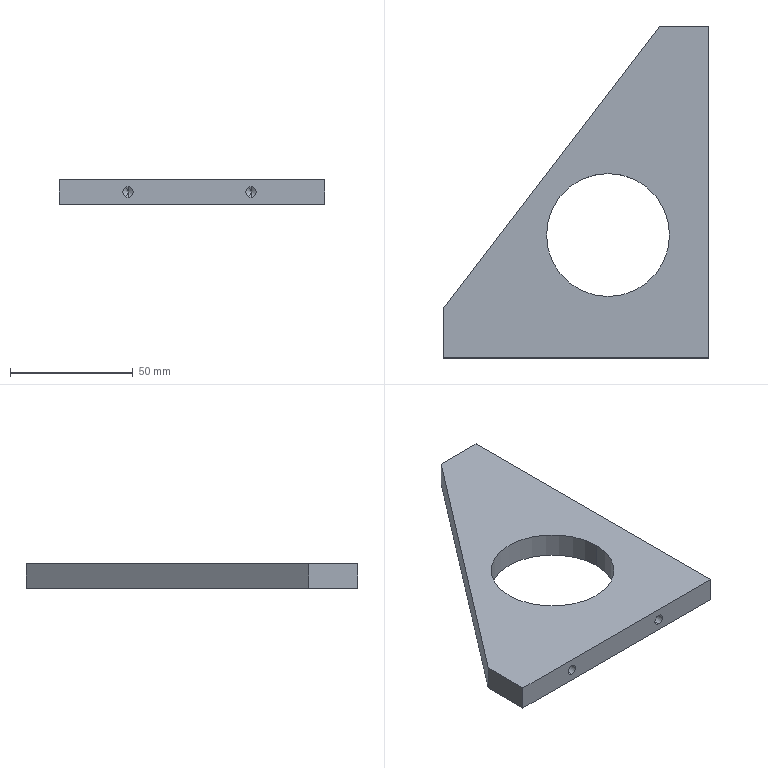Part | SolidWorks | features HoleWzd 2, ICE 2, Extrusion 1 | 1 solid | 25 faces | box 108 x 135 x 10 mm | volume 74855 mm3 | cylinder 10 | cone 8 | plane 7 | commonest cylinder face diameters 4.2 x8 50 x2
STEP:
#1=CARTESIAN_POINT('',(38.028,-17.5,10.));
#2=VERTEX_POINT('',#1);
#3=CARTESIAN_POINT('',(-11.972,-17.5,10.));
#4=VERTEX_POINT('',#3);
#5=CARTESIAN_POINT('',(13.028,-17.5,10.));
#6=DIRECTION('',(0.,0.,-1.));
#7=DIRECTION('',(1.,0.,0.));
#8=AXIS2_PLACEMENT_3D('',#5,#6,#7);
#9=CIRCLE('',#8,25.);
#10=EDGE_CURVE('',#2,#4,#9,.T.);
#11=ORIENTED_EDGE('',*,*,#10,.F.);
#12=CARTESIAN_POINT('',(38.028,-17.5,0.));
#13=VERTEX_POINT('',#12);
#14=CARTESIAN_POINT('',(38.028,-17.5,10.001));
#15=DIRECTION('',(0.,0.,-1.));
#16=VECTOR('',#15,1000.);
#17=LINE('',#14,#16);
#18=EDGE_CURVE('',#2,#13,#17,.T.);
#19=ORIENTED_EDGE('',*,*,#18,.T.);
#20=CARTESIAN_POINT('',(-11.972,-17.5,0.));
#21=VERTEX_POINT('',#20);
#22=CARTESIAN_POINT('',(13.028,-17.5,0.));
#23=DIRECTION('',(0.,0.,-1.));
#24=DIRECTION('',(-1.,0.,0.));
#25=AXIS2_PLACEMENT_3D('',#22,#23,#24);
#26=CIRCLE('',#25,25.);
#27=EDGE_CURVE('',#13,#21,#26,.T.);
#28=ORIENTED_EDGE('',*,*,#27,.T.);
#29=CARTESIAN_POINT('',(-11.972,-17.5,10.001));
#30=DIRECTION('',(0.,0.,-1.));
#31=VECTOR('',#30,1000.);
#32=LINE('',#29,#31);
#33=EDGE_CURVE('',#4,#21,#32,.T.);
#34=ORIENTED_EDGE('',*,*,#33,.F.);
#35=EDGE_LOOP('',(#11,#19,#28,#34));
#36=FACE_OUTER_BOUND('',#35,.T.);
#37=CARTESIAN_POINT('',(13.028,-17.5,10.001));
#38=DIRECTION('',(0.,0.,-1.));
#39=DIRECTION('',(-1.,0.,0.));
#40=AXIS2_PLACEMENT_3D('',#37,#38,#39);
#41=CYLINDRICAL_SURFACE('',#40,25.);
#42=ADVANCED_FACE('',(#36),#41,.F.);
#43=CARTESIAN_POINT('',(41.6,-27.5,7.1));
#44=VERTEX_POINT('',#43);
#45=CARTESIAN_POINT('',(41.6,-27.5,2.9));
#46=VERTEX_POINT('',#45);
#47=CARTESIAN_POINT('',(41.6,-27.5,5.));
#48=DIRECTION('',(1.,0.,0.));
#49=DIRECTION('',(0.,0.,-1.));
#50=AXIS2_PLACEMENT_3D('',#47,#48,#49);
#51=CIRCLE('',#50,2.1);
#52=EDGE_CURVE('',#44,#46,#51,.T.);
#53=ORIENTED_EDGE('',*,*,#52,.F.);
#54=CARTESIAN_POINT('',(54.,-27.5,7.1));
#55=VERTEX_POINT('',#54);
#56=CARTESIAN_POINT('',(54.,-27.5,7.1));
#57=DIRECTION('',(1.,0.,0.));
#58=VECTOR('',#57,1000.);
#59=LINE('',#56,#58);
#60=EDGE_CURVE('',#44,#55,#59,.T.);
#61=ORIENTED_EDGE('',*,*,#60,.T.);
#62=CARTESIAN_POINT('',(54.,-27.5,2.9));
#63=VERTEX_POINT('',#62);
#64=CARTESIAN_POINT('',(54.,-27.5,5.));
#65=DIRECTION('',(1.,0.,0.));
#66=DIRECTION('',(0.,0.,-1.));
#67=AXIS2_PLACEMENT_3D('',#64,#65,#66);
#68=CIRCLE('',#67,2.1);
#69=EDGE_CURVE('',#55,#63,#68,.T.);
#70=ORIENTED_EDGE('',*,*,#69,.T.);
#71=CARTESIAN_POINT('',(54.,-27.5,2.9));
#72=DIRECTION('',(1.,0.,0.));
#73=VECTOR('',#72,1000.);
#74=LINE('',#71,#73);
#75=EDGE_CURVE('',#46,#63,#74,.T.);
#76=ORIENTED_EDGE('',*,*,#75,.F.);
#77=EDGE_LOOP('',(#53,#61,#70,#76));
#78=FACE_OUTER_BOUND('',#77,.T.);
#79=CARTESIAN_POINT('',(54.,-27.5,5.));
#80=DIRECTION('',(1.,0.,0.));
#81=DIRECTION('',(0.,0.,-1.));
#82=AXIS2_PLACEMENT_3D('',#79,#80,#81);
#83=CYLINDRICAL_SURFACE('',#82,2.1);
#84=ADVANCED_FACE('',(#78),#83,.F.);
#85=CARTESIAN_POINT('',(40.338,-27.5,5.));
#86=VERTEX_POINT('',#85);
#87=CARTESIAN_POINT('',(41.6,-27.5,2.9));
#88=DIRECTION('',(0.515,0.,-0.8572));
#89=VECTOR('',#88,1000.);
#90=LINE('',#87,#89);
#91=EDGE_CURVE('',#86,#46,#90,.T.);
#92=ORIENTED_EDGE('',*,*,#91,.F.);
#93=CARTESIAN_POINT('',(41.6,-27.5,7.1));
#94=DIRECTION('',(0.515,0.,0.8572));
#95=VECTOR('',#94,1000.);
#96=LINE('',#93,#95);
#97=EDGE_CURVE('',#86,#44,#96,.T.);
#98=ORIENTED_EDGE('',*,*,#97,.T.);
#99=ORIENTED_EDGE('',*,*,#52,.T.);
#100=EDGE_LOOP('',(#92,#98,#99));
#101=FACE_OUTER_BOUND('',#100,.T.);
#102=CARTESIAN_POINT('',(41.6,-27.5,5.));
#103=DIRECTION('',(1.,0.,0.));
#104=DIRECTION('',(0.,0.,-1.));
#105=AXIS2_PLACEMENT_3D('',#102,#103,#104);
#106=CONICAL_SURFACE('',#105,2.1,1.03);
#107=ADVANCED_FACE('',(#101),#106,.F.);
#108=CARTESIAN_POINT('',(41.6,32.5,7.1));
#109=VERTEX_POINT('',#108);
#110=CARTESIAN_POINT('',(41.6,32.5,2.9));
#111=VERTEX_POINT('',#110);
#112=CARTESIAN_POINT('',(41.6,32.5,5.));
#113=DIRECTION('',(1.,0.,0.));
#114=DIRECTION('',(0.,0.,-1.));
#115=AXIS2_PLACEMENT_3D('',#112,#113,#114);
#116=CIRCLE('',#115,2.1);
#117=EDGE_CURVE('',#109,#111,#116,.T.);
#118=ORIENTED_EDGE('',*,*,#117,.F.);
#119=CARTESIAN_POINT('',(54.,32.5,7.1));
#120=VERTEX_POINT('',#119);
#121=CARTESIAN_POINT('',(54.,32.5,7.1));
#122=DIRECTION('',(1.,0.,0.));
#123=VECTOR('',#122,1000.);
#124=LINE('',#121,#123);
#125=EDGE_CURVE('',#109,#120,#124,.T.);
#126=ORIENTED_EDGE('',*,*,#125,.T.);
#127=CARTESIAN_POINT('',(54.,32.5,2.9));
#128=VERTEX_POINT('',#127);
#129=CARTESIAN_POINT('',(54.,32.5,5.));
#130=DIRECTION('',(1.,0.,0.));
#131=DIRECTION('',(0.,0.,-1.));
#132=AXIS2_PLACEMENT_3D('',#129,#130,#131);
#133=CIRCLE('',#132,2.1);
#134=EDGE_CURVE('',#120,#128,#133,.T.);
#135=ORIENTED_EDGE('',*,*,#134,.T.);
#136=CARTESIAN_POINT('',(54.,32.5,2.9));
#137=DIRECTION('',(1.,0.,0.));
#138=VECTOR('',#137,1000.);
#139=LINE('',#136,#138);
#140=EDGE_CURVE('',#111,#128,#139,.T.);
#141=ORIENTED_EDGE('',*,*,#140,.F.);
#142=EDGE_LOOP('',(#118,#126,#135,#141));
#143=FACE_OUTER_BOUND('',#142,.T.);
#144=CARTESIAN_POINT('',(54.,32.5,5.));
#145=DIRECTION('',(1.,0.,0.));
#146=DIRECTION('',(0.,0.,-1.));
#147=AXIS2_PLACEMENT_3D('',#144,#145,#146);
#148=CYLINDRICAL_SURFACE('',#147,2.1);
#149=ADVANCED_FACE('',(#143),#148,.F.);
#150=CARTESIAN_POINT('',(40.338,32.5,5.));
#151=VERTEX_POINT('',#150);
#152=CARTESIAN_POINT('',(41.6,32.5,2.9));
#153=DIRECTION('',(0.515,0.,-0.8572));
#154=VECTOR('',#153,1000.);
#155=LINE('',#152,#154);
#156=EDGE_CURVE('',#151,#111,#155,.T.);
#157=ORIENTED_EDGE('',*,*,#156,.F.);
#158=CARTESIAN_POINT('',(41.6,32.5,7.1));
#159=DIRECTION('',(0.515,0.,0.8572));
#160=VECTOR('',#159,1000.);
#161=LINE('',#158,#160);
#162=EDGE_CURVE('',#151,#109,#161,.T.);
#163=ORIENTED_EDGE('',*,*,#162,.T.);
#164=ORIENTED_EDGE('',*,*,#117,.T.);
#165=EDGE_LOOP('',(#157,#163,#164));
#166=FACE_OUTER_BOUND('',#165,.T.);
#167=CARTESIAN_POINT('',(41.6,32.5,5.));
#168=DIRECTION('',(1.,0.,0.));
#169=DIRECTION('',(0.,0.,-1.));
#170=AXIS2_PLACEMENT_3D('',#167,#168,#169);
#171=CONICAL_SURFACE('',#170,2.1,1.03);
#172=ADVANCED_FACE('',(#166),#171,.F.);
#173=CARTESIAN_POINT('',(24.,-55.1,7.1));
#174=VERTEX_POINT('',#173);
#175=CARTESIAN_POINT('',(24.,-55.1,2.9));
#176=VERTEX_POINT('',#175);
#177=CARTESIAN_POINT('',(24.,-55.1,5.));
#178=DIRECTION('',(0.,-1.,0.));
#179=DIRECTION('',(0.,0.,-1.));
#180=AXIS2_PLACEMENT_3D('',#177,#178,#179);
#181=CIRCLE('',#180,2.1);
#182=EDGE_CURVE('',#174,#176,#181,.T.);
#183=ORIENTED_EDGE('',*,*,#182,.F.);
#184=CARTESIAN_POINT('',(24.,-67.5,7.1));
#185=VERTEX_POINT('',#184);
#186=CARTESIAN_POINT('',(24.,-67.5,7.1));
#187=DIRECTION('',(0.,-1.,0.));
#188=VECTOR('',#187,1000.);
#189=LINE('',#186,#188);
#190=EDGE_CURVE('',#174,#185,#189,.T.);
#191=ORIENTED_EDGE('',*,*,#190,.T.);
#192=CARTESIAN_POINT('',(24.,-67.5,2.9));
#193=VERTEX_POINT('',#192);
#194=CARTESIAN_POINT('',(24.,-67.5,5.));
#195=DIRECTION('',(0.,-1.,0.));
#196=DIRECTION('',(0.,0.,-1.));
#197=AXIS2_PLACEMENT_3D('',#194,#195,#196);
#198=CIRCLE('',#197,2.1);
#199=EDGE_CURVE('',#185,#193,#198,.T.);
#200=ORIENTED_EDGE('',*,*,#199,.T.);
#201=CARTESIAN_POINT('',(24.,-67.5,2.9));
#202=DIRECTION('',(0.,-1.,0.));
#203=VECTOR('',#202,1000.);
#204=LINE('',#201,#203);
#205=EDGE_CURVE('',#176,#193,#204,.T.);
#206=ORIENTED_EDGE('',*,*,#205,.F.);
#207=EDGE_LOOP('',(#183,#191,#200,#206));
#208=FACE_OUTER_BOUND('',#207,.T.);
#209=CARTESIAN_POINT('',(24.,-67.5,5.));
#210=DIRECTION('',(0.,-1.,0.));
#211=DIRECTION('',(0.,0.,-1.));
#212=AXIS2_PLACEMENT_3D('',#209,#210,#211);
#213=CYLINDRICAL_SURFACE('',#212,2.1);
#214=ADVANCED_FACE('',(#208),#213,.F.);
#215=CARTESIAN_POINT('',(24.,-53.838,5.));
#216=VERTEX_POINT('',#215);
#217=CARTESIAN_POINT('',(24.,-55.1,2.9));
#218=DIRECTION('',(0.,-0.515,-0.8572));
#219=VECTOR('',#218,1000.);
#220=LINE('',#217,#219);
#221=EDGE_CURVE('',#216,#176,#220,.T.);
#222=ORIENTED_EDGE('',*,*,#221,.F.);
#223=CARTESIAN_POINT('',(24.,-55.1,7.1));
#224=DIRECTION('',(0.,-0.515,0.8572));
#225=VECTOR('',#224,1000.);
#226=LINE('',#223,#225);
#227=EDGE_CURVE('',#216,#174,#226,.T.);
#228=ORIENTED_EDGE('',*,*,#227,.T.);
#229=ORIENTED_EDGE('',*,*,#182,.T.);
#230=EDGE_LOOP('',(#222,#228,#229));
#231=FACE_OUTER_BOUND('',#230,.T.);
#232=CARTESIAN_POINT('',(24.,-55.1,5.));
#233=DIRECTION('',(0.,-1.,0.));
#234=DIRECTION('',(0.,0.,-1.));
#235=AXIS2_PLACEMENT_3D('',#232,#233,#234);
#236=CONICAL_SURFACE('',#235,2.1,1.03);
#237=ADVANCED_FACE('',(#231),#236,.F.);
#238=CARTESIAN_POINT('',(-26.,-55.1,7.1));
#239=VERTEX_POINT('',#238);
#240=CARTESIAN_POINT('',(-26.,-55.1,2.9));
#241=VERTEX_POINT('',#240);
#242=CARTESIAN_POINT('',(-26.,-55.1,5.));
#243=DIRECTION('',(0.,-1.,0.));
#244=DIRECTION('',(0.,0.,-1.));
#245=AXIS2_PLACEMENT_3D('',#242,#243,#244);
#246=CIRCLE('',#245,2.1);
#247=EDGE_CURVE('',#239,#241,#246,.T.);
#248=ORIENTED_EDGE('',*,*,#247,.F.);
#249=CARTESIAN_POINT('',(-26.,-67.5,7.1));
#250=VERTEX_POINT('',#249);
#251=CARTESIAN_POINT('',(-26.,-67.5,7.1));
#252=DIRECTION('',(0.,-1.,0.));
#253=VECTOR('',#252,1000.);
#254=LINE('',#251,#253);
#255=EDGE_CURVE('',#239,#250,#254,.T.);
#256=ORIENTED_EDGE('',*,*,#255,.T.);
#257=CARTESIAN_POINT('',(-26.,-67.5,2.9));
#258=VERTEX_POINT('',#257);
#259=CARTESIAN_POINT('',(-26.,-67.5,5.));
#260=DIRECTION('',(0.,-1.,0.));
#261=DIRECTION('',(0.,0.,-1.));
#262=AXIS2_PLACEMENT_3D('',#259,#260,#261);
#263=CIRCLE('',#262,2.1);
#264=EDGE_CURVE('',#250,#258,#263,.T.);
#265=ORIENTED_EDGE('',*,*,#264,.T.);
#266=CARTESIAN_POINT('',(-26.,-67.5,2.9));
#267=DIRECTION('',(0.,-1.,0.));
#268=VECTOR('',#267,1000.);
#269=LINE('',#266,#268);
#270=EDGE_CURVE('',#241,#258,#269,.T.);
#271=ORIENTED_EDGE('',*,*,#270,.F.);
#272=EDGE_LOOP('',(#248,#256,#265,#271));
#273=FACE_OUTER_BOUND('',#272,.T.);
#274=CARTESIAN_POINT('',(-26.,-67.5,5.));
#275=DIRECTION('',(0.,-1.,0.));
#276=DIRECTION('',(0.,0.,-1.));
#277=AXIS2_PLACEMENT_3D('',#274,#275,#276);
#278=CYLINDRICAL_SURFACE('',#277,2.1);
#279=ADVANCED_FACE('',(#273),#278,.F.);
#280=CARTESIAN_POINT('',(-26.,-53.838,5.));
#281=VERTEX_POINT('',#280);
#282=CARTESIAN_POINT('',(-26.,-55.1,2.9));
#283=DIRECTION('',(0.,-0.515,-0.8572));
#284=VECTOR('',#283,1000.);
#285=LINE('',#282,#284);
#286=EDGE_CURVE('',#281,#241,#285,.T.);
#287=ORIENTED_EDGE('',*,*,#286,.F.);
#288=CARTESIAN_POINT('',(-26.,-55.1,7.1));
#289=DIRECTION('',(0.,-0.515,0.8572));
#290=VECTOR('',#289,1000.);
#291=LINE('',#288,#290);
#292=EDGE_CURVE('',#281,#239,#291,.T.);
#293=ORIENTED_EDGE('',*,*,#292,.T.);
#294=ORIENTED_EDGE('',*,*,#247,.T.);
#295=EDGE_LOOP('',(#287,#293,#294));
#296=FACE_OUTER_BOUND('',#295,.T.);
#297=CARTESIAN_POINT('',(-26.,-55.1,5.));
#298=DIRECTION('',(0.,-1.,0.));
#299=DIRECTION('',(0.,0.,-1.));
#300=AXIS2_PLACEMENT_3D('',#297,#298,#299);
#301=CONICAL_SURFACE('',#300,2.1,1.03);
#302=ADVANCED_FACE('',(#296),#301,.F.);
#303=CARTESIAN_POINT('',(-54.,-47.5,10.));
#304=VERTEX_POINT('',#303);
#305=CARTESIAN_POINT('',(-54.,-67.5,10.));
#306=VERTEX_POINT('',#305);
#307=CARTESIAN_POINT('',(-54.,-67.5,10.));
#308=DIRECTION('',(0.,-1.,0.));
#309=VECTOR('',#308,1000.);
#310=LINE('',#307,#309);
#311=EDGE_CURVE('',#304,#306,#310,.T.);
#312=ORIENTED_EDGE('',*,*,#311,.F.);
#313=CARTESIAN_POINT('',(-54.,-47.5,0.));
#314=VERTEX_POINT('',#313);
#315=CARTESIAN_POINT('',(-54.,-47.5,-0.001));
#316=DIRECTION('',(0.,0.,1.));
#317=VECTOR('',#316,1000.);
#318=LINE('',#315,#317);
#319=EDGE_CURVE('',#314,#304,#318,.T.);
#320=ORIENTED_EDGE('',*,*,#319,.F.);
#321=CARTESIAN_POINT('',(-54.,-67.5,0.));
#322=VERTEX_POINT('',#321);
#323=CARTESIAN_POINT('',(-54.,-67.5,0.));
#324=DIRECTION('',(0.,-1.,0.));
#325=VECTOR('',#324,1000.);
#326=LINE('',#323,#325);
#327=EDGE_CURVE('',#314,#322,#326,.T.);
#328=ORIENTED_EDGE('',*,*,#327,.T.);
#329=CARTESIAN_POINT('',(-54.,-67.5,10.));
#330=DIRECTION('',(0.,0.,-1.));
#331=VECTOR('',#330,1000.);
#332=LINE('',#329,#331);
#333=EDGE_CURVE('',#306,#322,#332,.T.);
#334=ORIENTED_EDGE('',*,*,#333,.F.);
#335=EDGE_LOOP('',(#312,#320,#328,#334));
#336=FACE_OUTER_BOUND('',#335,.T.);
#337=CARTESIAN_POINT('',(-54.,-67.5,10.));
#338=DIRECTION('',(1.,0.,0.));
#339=DIRECTION('',(0.,0.,-1.));
#340=AXIS2_PLACEMENT_3D('',#337,#338,#339);
#341=PLANE('',#340);
#342=ADVANCED_FACE('',(#336),#341,.F.);
#343=CARTESIAN_POINT('',(24.,-67.5,5.));
#344=DIRECTION('',(0.,-1.,0.));
#345=DIRECTION('',(0.,0.,-1.));
#346=AXIS2_PLACEMENT_3D('',#343,#344,#345);
#347=CIRCLE('',#346,2.1);
#348=EDGE_CURVE('',#193,#185,#347,.T.);
#349=ORIENTED_EDGE('',*,*,#348,.F.);
#350=ORIENTED_EDGE('',*,*,#199,.F.);
#351=EDGE_LOOP('',(#349,#350));
#352=FACE_BOUND('',#351,.T.);
#353=CARTESIAN_POINT('',(-26.,-67.5,5.));
#354=DIRECTION('',(0.,-1.,0.));
#355=DIRECTION('',(0.,0.,-1.));
#356=AXIS2_PLACEMENT_3D('',#353,#354,#355);
#357=CIRCLE('',#356,2.1);
#358=EDGE_CURVE('',#258,#250,#357,.T.);
#359=ORIENTED_EDGE('',*,*,#358,.F.);
#360=ORIENTED_EDGE('',*,*,#264,.F.);
#361=EDGE_LOOP('',(#359,#360));
#362=FACE_BOUND('',#361,.T.);
#363=CARTESIAN_POINT('',(54.,-67.5,0.));
#364=VERTEX_POINT('',#363);
#365=CARTESIAN_POINT('',(54.,-67.5,0.));
#366=DIRECTION('',(1.,0.,0.));
#367=VECTOR('',#366,1000.);
#368=LINE('',#365,#367);
#369=EDGE_CURVE('',#322,#364,#368,.T.);
#370=ORIENTED_EDGE('',*,*,#369,.T.);
#371=CARTESIAN_POINT('',(54.,-67.5,10.));
#372=VERTEX_POINT('',#371);
#373=CARTESIAN_POINT('',(54.,-67.5,10.));
#374=DIRECTION('',(0.,0.,-1.));
#375=VECTOR('',#374,1000.);
#376=LINE('',#373,#375);
#377=EDGE_CURVE('',#372,#364,#376,.T.);
#378=ORIENTED_EDGE('',*,*,#377,.F.);
#379=CARTESIAN_POINT('',(54.,-67.5,10.));
#380=DIRECTION('',(1.,0.,0.));
#381=VECTOR('',#380,1000.);
#382=LINE('',#379,#381);
#383=EDGE_CURVE('',#306,#372,#382,.T.);
#384=ORIENTED_EDGE('',*,*,#383,.F.);
#385=ORIENTED_EDGE('',*,*,#333,.T.);
#386=EDGE_LOOP('',(#370,#378,#384,#385));
#387=FACE_OUTER_BOUND('',#386,.T.);
#388=CARTESIAN_POINT('',(54.,-67.5,10.));
#389=DIRECTION('',(0.,1.,0.));
#390=DIRECTION('',(-1.,0.,0.));
#391=AXIS2_PLACEMENT_3D('',#388,#389,#390);
#392=PLANE('',#391);
#393=ADVANCED_FACE('',(#352,#362,#387),#392,.F.);
#394=CARTESIAN_POINT('',(54.,-27.5,5.));
#395=DIRECTION('',(1.,0.,0.));
#396=DIRECTION('',(0.,0.,-1.));
#397=AXIS2_PLACEMENT_3D('',#394,#395,#396);
#398=CIRCLE('',#397,2.1);
#399=EDGE_CURVE('',#63,#55,#398,.T.);
#400=ORIENTED_EDGE('',*,*,#399,.F.);
#401=ORIENTED_EDGE('',*,*,#69,.F.);
#402=EDGE_LOOP('',(#400,#401));
#403=FACE_BOUND('',#402,.T.);
#404=CARTESIAN_POINT('',(54.,32.5,5.));
#405=DIRECTION('',(1.,0.,0.));
#406=DIRECTION('',(0.,0.,-1.));
#407=AXIS2_PLACEMENT_3D('',#404,#405,#406);
#408=CIRCLE('',#407,2.1);
#409=EDGE_CURVE('',#128,#120,#408,.T.);
#410=ORIENTED_EDGE('',*,*,#409,.F.);
#411=ORIENTED_EDGE('',*,*,#134,.F.);
#412=EDGE_LOOP('',(#410,#411));
#413=FACE_BOUND('',#412,.T.);
#414=CARTESIAN_POINT('',(54.,67.5,0.));
#415=VERTEX_POINT('',#414);
#416=CARTESIAN_POINT('',(54.,-67.5,0.));
#417=DIRECTION('',(0.,1.,0.));
#418=VECTOR('',#417,1000.);
#419=LINE('',#416,#418);
#420=EDGE_CURVE('',#364,#415,#419,.T.);
#421=ORIENTED_EDGE('',*,*,#420,.T.);
#422=CARTESIAN_POINT('',(54.,67.5,10.));
#423=VERTEX_POINT('',#422);
#424=CARTESIAN_POINT('',(54.,67.5,10.));
#425=DIRECTION('',(0.,0.,-1.));
#426=VECTOR('',#425,1000.);
#427=LINE('',#424,#426);
#428=EDGE_CURVE('',#423,#415,#427,.T.);
#429=ORIENTED_EDGE('',*,*,#428,.F.);
#430=CARTESIAN_POINT('',(54.,-67.5,10.));
#431=DIRECTION('',(0.,1.,0.));
#432=VECTOR('',#431,1000.);
#433=LINE('',#430,#432);
#434=EDGE_CURVE('',#372,#423,#433,.T.);
#435=ORIENTED_EDGE('',*,*,#434,.F.);
#436=ORIENTED_EDGE('',*,*,#377,.T.);
#437=EDGE_LOOP('',(#421,#429,#435,#436));
#438=FACE_OUTER_BOUND('',#437,.T.);
#439=CARTESIAN_POINT('',(54.,-67.5,10.));
#440=DIRECTION('',(-1.,0.,0.));
#441=DIRECTION('',(0.,0.,1.));
#442=AXIS2_PLACEMENT_3D('',#439,#440,#441);
#443=PLANE('',#442);
#444=ADVANCED_FACE('',(#403,#413,#438),#443,.F.);
#445=CARTESIAN_POINT('',(34.,67.5,0.));
#446=VERTEX_POINT('',#445);
#447=CARTESIAN_POINT('',(54.,67.5,0.));
#448=DIRECTION('',(-1.,0.,0.));
#449=VECTOR('',#448,1000.);
#450=LINE('',#447,#449);
#451=EDGE_CURVE('',#415,#446,#450,.T.);
#452=ORIENTED_EDGE('',*,*,#451,.T.);
#453=CARTESIAN_POINT('',(34.,67.5,10.));
#454=VERTEX_POINT('',#453);
#455=CARTESIAN_POINT('',(34.,67.5,-0.001));
#456=DIRECTION('',(0.,0.,1.));
#457=VECTOR('',#456,1000.);
#458=LINE('',#455,#457);
#459=EDGE_CURVE('',#446,#454,#458,.T.);
#460=ORIENTED_EDGE('',*,*,#459,.T.);
#461=CARTESIAN_POINT('',(54.,67.5,10.));
#462=DIRECTION('',(-1.,0.,0.));
#463=VECTOR('',#462,1000.);
#464=LINE('',#461,#463);
#465=EDGE_CURVE('',#423,#454,#464,.T.);
#466=ORIENTED_EDGE('',*,*,#465,.F.);
#467=ORIENTED_EDGE('',*,*,#428,.T.);
#468=EDGE_LOOP('',(#452,#460,#466,#467));
#469=FACE_OUTER_BOUND('',#468,.T.);
#470=CARTESIAN_POINT('',(54.,67.5,10.));
#471=DIRECTION('',(0.,-1.,0.));
#472=DIRECTION('',(1.,0.,0.));
#473=AXIS2_PLACEMENT_3D('',#470,#471,#472);
#474=PLANE('',#473);
#475=ADVANCED_FACE('',(#469),#474,.F.);
#476=CARTESIAN_POINT('',(13.028,-17.5,10.));
#477=DIRECTION('',(0.,0.,-1.));
#478=DIRECTION('',(1.,0.,0.));
#479=AXIS2_PLACEMENT_3D('',#476,#477,#478);
#480=CIRCLE('',#479,25.);
#481=EDGE_CURVE('',#4,#2,#480,.T.);
#482=ORIENTED_EDGE('',*,*,#481,.T.);
#483=ORIENTED_EDGE('',*,*,#10,.T.);
#484=EDGE_LOOP('',(#482,#483));
#485=FACE_BOUND('',#484,.T.);
#486=CARTESIAN_POINT('',(-54.,-47.5,10.));
#487=DIRECTION('',(0.6077,0.7942,0.));
#488=VECTOR('',#487,1000.);
#489=LINE('',#486,#488);
#490=EDGE_CURVE('',#304,#454,#489,.T.);
#491=ORIENTED_EDGE('',*,*,#490,.F.);
#492=ORIENTED_EDGE('',*,*,#311,.T.);
#493=ORIENTED_EDGE('',*,*,#383,.T.);
#494=ORIENTED_EDGE('',*,*,#434,.T.);
#495=ORIENTED_EDGE('',*,*,#465,.T.);
#496=EDGE_LOOP('',(#491,#492,#493,#494,#495));
#497=FACE_OUTER_BOUND('',#496,.T.);
#498=CARTESIAN_POINT('',(0.,0.,10.));
#499=DIRECTION('',(0.,0.,1.));
#500=DIRECTION('',(1.,0.,0.));
#501=AXIS2_PLACEMENT_3D('',#498,#499,#500);
#502=PLANE('',#501);
#503=ADVANCED_FACE('',(#485,#497),#502,.T.);
#504=CARTESIAN_POINT('',(13.028,-17.5,0.));
#505=DIRECTION('',(0.,0.,-1.));
#506=DIRECTION('',(-1.,0.,0.));
#507=AXIS2_PLACEMENT_3D('',#504,#505,#506);
#508=CIRCLE('',#507,25.);
#509=EDGE_CURVE('',#21,#13,#508,.T.);
#510=ORIENTED_EDGE('',*,*,#509,.F.);
#511=ORIENTED_EDGE('',*,*,#27,.F.);
#512=EDGE_LOOP('',(#510,#511));
#513=FACE_BOUND('',#512,.T.);
#514=ORIENTED_EDGE('',*,*,#327,.F.);
#515=CARTESIAN_POINT('',(-54.,-47.5,0.));
#516=DIRECTION('',(-0.6077,-0.7942,0.));
#517=VECTOR('',#516,1000.);
#518=LINE('',#515,#517);
#519=EDGE_CURVE('',#446,#314,#518,.T.);
#520=ORIENTED_EDGE('',*,*,#519,.F.);
#521=ORIENTED_EDGE('',*,*,#451,.F.);
#522=ORIENTED_EDGE('',*,*,#420,.F.);
#523=ORIENTED_EDGE('',*,*,#369,.F.);
#524=EDGE_LOOP('',(#514,#520,#521,#522,#523));
#525=FACE_OUTER_BOUND('',#524,.T.);
#526=CARTESIAN_POINT('',(0.,0.,0.));
#527=DIRECTION('',(0.,0.,1.));
#528=DIRECTION('',(1.,0.,0.));
#529=AXIS2_PLACEMENT_3D('',#526,#527,#528);
#530=PLANE('',#529);
#531=ADVANCED_FACE('',(#513,#525),#530,.F.);
#532=ORIENTED_EDGE('',*,*,#519,.T.);
#533=ORIENTED_EDGE('',*,*,#319,.T.);
#534=ORIENTED_EDGE('',*,*,#490,.T.);
#535=ORIENTED_EDGE('',*,*,#459,.F.);
#536=EDGE_LOOP('',(#532,#533,#534,#535));
#537=FACE_OUTER_BOUND('',#536,.T.);
#538=CARTESIAN_POINT('',(-54.,-47.5,-0.001));
#539=DIRECTION('',(0.7942,-0.6077,0.));
#540=DIRECTION('',(0.6077,0.7942,0.));
#541=AXIS2_PLACEMENT_3D('',#538,#539,#540);
#542=PLANE('',#541);
#543=ADVANCED_FACE('',(#537),#542,.F.);
#544=ORIENTED_EDGE('',*,*,#292,.F.);
#545=ORIENTED_EDGE('',*,*,#286,.T.);
#546=CARTESIAN_POINT('',(-26.,-55.1,5.));
#547=DIRECTION('',(0.,-1.,0.));
#548=DIRECTION('',(0.,0.,-1.));
#549=AXIS2_PLACEMENT_3D('',#546,#547,#548);
#550=CIRCLE('',#549,2.1);
#551=EDGE_CURVE('',#241,#239,#550,.T.);
#552=ORIENTED_EDGE('',*,*,#551,.T.);
#553=EDGE_LOOP('',(#544,#545,#552));
#554=FACE_OUTER_BOUND('',#553,.T.);
#555=CARTESIAN_POINT('',(-26.,-55.1,5.));
#556=DIRECTION('',(0.,-1.,0.));
#557=DIRECTION('',(0.,0.,-1.));
#558=AXIS2_PLACEMENT_3D('',#555,#556,#557);
#559=CONICAL_SURFACE('',#558,2.1,1.03);
#560=ADVANCED_FACE('',(#554),#559,.F.);
#561=ORIENTED_EDGE('',*,*,#255,.F.);
#562=ORIENTED_EDGE('',*,*,#551,.F.);
#563=ORIENTED_EDGE('',*,*,#270,.T.);
#564=ORIENTED_EDGE('',*,*,#358,.T.);
#565=EDGE_LOOP('',(#561,#562,#563,#564));
#566=FACE_OUTER_BOUND('',#565,.T.);
#567=CARTESIAN_POINT('',(-26.,-67.5,5.));
#568=DIRECTION('',(0.,-1.,0.));
#569=DIRECTION('',(0.,0.,-1.));
#570=AXIS2_PLACEMENT_3D('',#567,#568,#569);
#571=CYLINDRICAL_SURFACE('',#570,2.1);
#572=ADVANCED_FACE('',(#566),#571,.F.);
#573=ORIENTED_EDGE('',*,*,#227,.F.);
#574=ORIENTED_EDGE('',*,*,#221,.T.);
#575=CARTESIAN_POINT('',(24.,-55.1,5.));
#576=DIRECTION('',(0.,-1.,0.));
#577=DIRECTION('',(0.,0.,-1.));
#578=AXIS2_PLACEMENT_3D('',#575,#576,#577);
#579=CIRCLE('',#578,2.1);
#580=EDGE_CURVE('',#176,#174,#579,.T.);
#581=ORIENTED_EDGE('',*,*,#580,.T.);
#582=EDGE_LOOP('',(#573,#574,#581));
#583=FACE_OUTER_BOUND('',#582,.T.);
#584=CARTESIAN_POINT('',(24.,-55.1,5.));
#585=DIRECTION('',(0.,-1.,0.));
#586=DIRECTION('',(0.,0.,-1.));
#587=AXIS2_PLACEMENT_3D('',#584,#585,#586);
#588=CONICAL_SURFACE('',#587,2.1,1.03);
#589=ADVANCED_FACE('',(#583),#588,.F.);
#590=ORIENTED_EDGE('',*,*,#190,.F.);
#591=ORIENTED_EDGE('',*,*,#580,.F.);
#592=ORIENTED_EDGE('',*,*,#205,.T.);
#593=ORIENTED_EDGE('',*,*,#348,.T.);
#594=EDGE_LOOP('',(#590,#591,#592,#593));
#595=FACE_OUTER_BOUND('',#594,.T.);
#596=CARTESIAN_POINT('',(24.,-67.5,5.));
#597=DIRECTION('',(0.,-1.,0.));
#598=DIRECTION('',(0.,0.,-1.));
#599=AXIS2_PLACEMENT_3D('',#596,#597,#598);
#600=CYLINDRICAL_SURFACE('',#599,2.1);
#601=ADVANCED_FACE('',(#595),#600,.F.);
#602=ORIENTED_EDGE('',*,*,#162,.F.);
#603=ORIENTED_EDGE('',*,*,#156,.T.);
#604=CARTESIAN_POINT('',(41.6,32.5,5.));
#605=DIRECTION('',(1.,0.,0.));
#606=DIRECTION('',(0.,0.,-1.));
#607=AXIS2_PLACEMENT_3D('',#604,#605,#606);
#608=CIRCLE('',#607,2.1);
#609=EDGE_CURVE('',#111,#109,#608,.T.);
#610=ORIENTED_EDGE('',*,*,#609,.T.);
#611=EDGE_LOOP('',(#602,#603,#610));
#612=FACE_OUTER_BOUND('',#611,.T.);
#613=CARTESIAN_POINT('',(41.6,32.5,5.));
#614=DIRECTION('',(1.,0.,0.));
#615=DIRECTION('',(0.,0.,-1.));
#616=AXIS2_PLACEMENT_3D('',#613,#614,#615);
#617=CONICAL_SURFACE('',#616,2.1,1.03);
#618=ADVANCED_FACE('',(#612),#617,.F.);
#619=ORIENTED_EDGE('',*,*,#125,.F.);
#620=ORIENTED_EDGE('',*,*,#609,.F.);
#621=ORIENTED_EDGE('',*,*,#140,.T.);
#622=ORIENTED_EDGE('',*,*,#409,.T.);
#623=EDGE_LOOP('',(#619,#620,#621,#622));
#624=FACE_OUTER_BOUND('',#623,.T.);
#625=CARTESIAN_POINT('',(54.,32.5,5.));
#626=DIRECTION('',(1.,0.,0.));
#627=DIRECTION('',(0.,0.,-1.));
#628=AXIS2_PLACEMENT_3D('',#625,#626,#627);
#629=CYLINDRICAL_SURFACE('',#628,2.1);
#630=ADVANCED_FACE('',(#624),#629,.F.);
#631=ORIENTED_EDGE('',*,*,#97,.F.);
#632=ORIENTED_EDGE('',*,*,#91,.T.);
#633=CARTESIAN_POINT('',(41.6,-27.5,5.));
#634=DIRECTION('',(1.,0.,0.));
#635=DIRECTION('',(0.,0.,-1.));
#636=AXIS2_PLACEMENT_3D('',#633,#634,#635);
#637=CIRCLE('',#636,2.1);
#638=EDGE_CURVE('',#46,#44,#637,.T.);
#639=ORIENTED_EDGE('',*,*,#638,.T.);
#640=EDGE_LOOP('',(#631,#632,#639));
#641=FACE_OUTER_BOUND('',#640,.T.);
#642=CARTESIAN_POINT('',(41.6,-27.5,5.));
#643=DIRECTION('',(1.,0.,0.));
#644=DIRECTION('',(0.,0.,-1.));
#645=AXIS2_PLACEMENT_3D('',#642,#643,#644);
#646=CONICAL_SURFACE('',#645,2.1,1.03);
#647=ADVANCED_FACE('',(#641),#646,.F.);
#648=ORIENTED_EDGE('',*,*,#60,.F.);
#649=ORIENTED_EDGE('',*,*,#638,.F.);
#650=ORIENTED_EDGE('',*,*,#75,.T.);
#651=ORIENTED_EDGE('',*,*,#399,.T.);
#652=EDGE_LOOP('',(#648,#649,#650,#651));
#653=FACE_OUTER_BOUND('',#652,.T.);
#654=CARTESIAN_POINT('',(54.,-27.5,5.));
#655=DIRECTION('',(1.,0.,0.));
#656=DIRECTION('',(0.,0.,-1.));
#657=AXIS2_PLACEMENT_3D('',#654,#655,#656);
#658=CYLINDRICAL_SURFACE('',#657,2.1);
#659=ADVANCED_FACE('',(#653),#658,.F.);
#660=ORIENTED_EDGE('',*,*,#18,.F.);
#661=ORIENTED_EDGE('',*,*,#481,.F.);
#662=ORIENTED_EDGE('',*,*,#33,.T.);
#663=ORIENTED_EDGE('',*,*,#509,.T.);
#664=EDGE_LOOP('',(#660,#661,#662,#663));
#665=FACE_OUTER_BOUND('',#664,.T.);
#666=CARTESIAN_POINT('',(13.028,-17.5,10.001));
#667=DIRECTION('',(0.,0.,-1.));
#668=DIRECTION('',(-1.,0.,0.));
#669=AXIS2_PLACEMENT_3D('',#666,#667,#668);
#670=CYLINDRICAL_SURFACE('',#669,25.);
#671=ADVANCED_FACE('',(#665),#670,.F.);
#672=CLOSED_SHELL('',(#42,#84,#107,#149,#172,#214,#237,#279,#302,#342,#393,#444,#475,#503,#531,#543,#560,#572,#589,#601,#618,#630,#647,#659,#671));
#673=MANIFOLD_SOLID_BREP('',#672);
#674=CARTESIAN_POINT('',(0.,0.,0.));
#675=DIRECTION('',(0.,0.,1.));
#676=DIRECTION('',(1.,0.,0.));
#677=AXIS2_PLACEMENT_3D('',#674,#675,#676);
#678=(LENGTH_UNIT()NAMED_UNIT(*)SI_UNIT(.MILLI.,.METRE.));
#679=UNCERTAINTY_MEASURE_WITH_UNIT(LENGTH_MEASURE(0.00001),#678,'','');
#680=(NAMED_UNIT(*)PLANE_ANGLE_UNIT()SI_UNIT($,.RADIAN.));
#681=(NAMED_UNIT(*)SI_UNIT($,.STERADIAN.)SOLID_ANGLE_UNIT());
#682=(GEOMETRIC_REPRESENTATION_CONTEXT(3)GLOBAL_UNCERTAINTY_ASSIGNED_CONTEXT((#679))GLOBAL_UNIT_ASSIGNED_CONTEXT((#678,#680,#681))REPRESENTATION_CONTEXT('',''));
#683=ADVANCED_BREP_SHAPE_REPRESENTATION('',(#673,#677),#682);